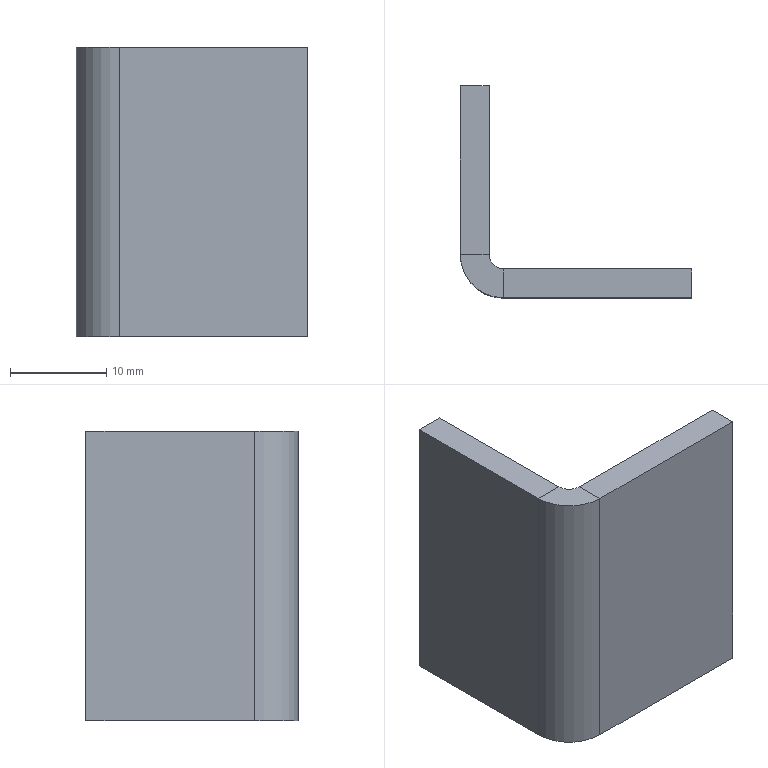Part | STEP file | 5091404 | 1 solid | 14 faces | box 24 x 22 x 30 mm | volume 3754 mm3 | plane 12 | cylinder 2 | commonest cylinder face diameters 3 x1 9 x1
STEP:
#1=CARTESIAN_POINT('',(0.,0.,0.));
#2=DIRECTION('',(0.,0.,1.));
#3=DIRECTION('',(1.,0.,0.));
#4=AXIS2_PLACEMENT_3D('',#1,#2,#3);
#5=CARTESIAN_POINT('',(0.,4.5,15.));
#6=VERTEX_POINT('',#5);
#7=CARTESIAN_POINT('',(3.,4.5,15.));
#8=VERTEX_POINT('',#7);
#9=CARTESIAN_POINT('',(0.,4.5,15.));
#10=DIRECTION('',(1.,0.,0.));
#11=VECTOR('',#10,1.);
#12=LINE('',#9,#11);
#13=CARTESIAN_POINT('',(0.,4.5,15.));
#14=DIRECTION('',(0.,0.,1.));
#15=DIRECTION('',(1.,0.,0.));
#16=AXIS2_PLACEMENT_3D('',#13,#14,#15);
#17=PLANE('',#16);
#18=CARTESIAN_POINT('',(0.,0.));
#19=DIRECTION('',(1.,0.));
#20=VECTOR('',#19,1.);
#21=LINE('',#18,#20);
#22=(GEOMETRIC_REPRESENTATION_CONTEXT(2)PARAMETRIC_REPRESENTATION_CONTEXT()REPRESENTATION_CONTEXT('',''));
#23=DEFINITIONAL_REPRESENTATION('',(#21),#22);
#24=PCURVE('',#17,#23);
#25=CARTESIAN_POINT('',(4.5,3.,15.));
#26=DIRECTION('',(0.,0.,1.));
#27=DIRECTION('',(1.,0.,0.));
#28=AXIS2_PLACEMENT_3D('',#25,#26,#27);
#29=PLANE('',#28);
#30=CARTESIAN_POINT('',(-4.5,1.5));
#31=DIRECTION('',(1.,0.));
#32=VECTOR('',#31,1.);
#33=LINE('',#30,#32);
#34=(GEOMETRIC_REPRESENTATION_CONTEXT(2)PARAMETRIC_REPRESENTATION_CONTEXT()REPRESENTATION_CONTEXT('',''));
#35=DEFINITIONAL_REPRESENTATION('',(#33),#34);
#36=PCURVE('',#29,#35);
#37=SURFACE_CURVE('',#12,(#24,#36),.PCURVE_S1.);
#38=EDGE_CURVE('',#6,#8,#37,.T.);
#39=ORIENTED_EDGE('',*,*,#38,.F.);
#40=CARTESIAN_POINT('',(4.5,0.,15.));
#41=VERTEX_POINT('',#40);
#42=CARTESIAN_POINT('',(4.5,4.5,15.));
#43=DIRECTION('',(0.,0.,1.));
#44=DIRECTION('',(-1.,0.,0.));
#45=AXIS2_PLACEMENT_3D('',#42,#43,#44);
#46=CIRCLE('',#45,4.5);
#47=CARTESIAN_POINT('',(4.5,0.));
#48=DIRECTION('',(-1.,0.));
#49=AXIS2_PLACEMENT_2D('',#47,#48);
#50=CIRCLE('',#49,4.5);
#51=(GEOMETRIC_REPRESENTATION_CONTEXT(2)PARAMETRIC_REPRESENTATION_CONTEXT()REPRESENTATION_CONTEXT('',''));
#52=DEFINITIONAL_REPRESENTATION('',(#50),#51);
#53=PCURVE('',#17,#52);
#54=CARTESIAN_POINT('',(4.5,4.5,15.));
#55=DIRECTION('',(0.,0.,-1.));
#56=DIRECTION('',(-1.,0.,0.));
#57=AXIS2_PLACEMENT_3D('',#54,#55,#56);
#58=CYLINDRICAL_SURFACE('',#57,4.5);
#59=CARTESIAN_POINT('',(6.283,0.));
#60=DIRECTION('',(-1.,0.));
#61=VECTOR('',#60,1.);
#62=LINE('',#59,#61);
#63=(GEOMETRIC_REPRESENTATION_CONTEXT(2)PARAMETRIC_REPRESENTATION_CONTEXT()REPRESENTATION_CONTEXT('',''));
#64=DEFINITIONAL_REPRESENTATION('',(#62),#63);
#65=PCURVE('',#58,#64);
#66=SURFACE_CURVE('',#46,(#53,#65),.PCURVE_S1.);
#67=EDGE_CURVE('',#6,#41,#66,.T.);
#68=ORIENTED_EDGE('',*,*,#67,.T.);
#69=CARTESIAN_POINT('',(4.5,3.,15.));
#70=VERTEX_POINT('',#69);
#71=CARTESIAN_POINT('',(4.5,3.,15.));
#72=DIRECTION('',(0.,-1.,0.));
#73=VECTOR('',#72,1.);
#74=LINE('',#71,#73);
#75=CARTESIAN_POINT('',(4.5,-1.5));
#76=DIRECTION('',(0.,-1.));
#77=VECTOR('',#76,1.);
#78=LINE('',#75,#77);
#79=(GEOMETRIC_REPRESENTATION_CONTEXT(2)PARAMETRIC_REPRESENTATION_CONTEXT()REPRESENTATION_CONTEXT('',''));
#80=DEFINITIONAL_REPRESENTATION('',(#78),#79);
#81=PCURVE('',#17,#80);
#82=CARTESIAN_POINT('',(4.5,4.5,15.));
#83=DIRECTION('',(0.,0.,1.));
#84=DIRECTION('',(1.,0.,0.));
#85=AXIS2_PLACEMENT_3D('',#82,#83,#84);
#86=PLANE('',#85);
#87=CARTESIAN_POINT('',(0.,-1.5));
#88=DIRECTION('',(0.,-1.));
#89=VECTOR('',#88,1.);
#90=LINE('',#87,#89);
#91=(GEOMETRIC_REPRESENTATION_CONTEXT(2)PARAMETRIC_REPRESENTATION_CONTEXT()REPRESENTATION_CONTEXT('',''));
#92=DEFINITIONAL_REPRESENTATION('',(#90),#91);
#93=PCURVE('',#86,#92);
#94=SURFACE_CURVE('',#74,(#81,#93),.PCURVE_S1.);
#95=EDGE_CURVE('',#70,#41,#94,.T.);
#96=ORIENTED_EDGE('',*,*,#95,.F.);
#97=CARTESIAN_POINT('',(4.5,4.5,15.));
#98=DIRECTION('',(0.,0.,1.));
#99=DIRECTION('',(1.,0.,0.));
#100=AXIS2_PLACEMENT_3D('',#97,#98,#99);
#101=CIRCLE('',#100,1.5);
#102=CARTESIAN_POINT('',(4.5,0.));
#103=DIRECTION('',(1.,0.));
#104=AXIS2_PLACEMENT_2D('',#102,#103);
#105=CIRCLE('',#104,1.5);
#106=(GEOMETRIC_REPRESENTATION_CONTEXT(2)PARAMETRIC_REPRESENTATION_CONTEXT()REPRESENTATION_CONTEXT('',''));
#107=DEFINITIONAL_REPRESENTATION('',(#105),#106);
#108=PCURVE('',#17,#107);
#109=CARTESIAN_POINT('',(4.5,4.5,15.));
#110=DIRECTION('',(0.,0.,-1.));
#111=DIRECTION('',(-1.,0.,0.));
#112=AXIS2_PLACEMENT_3D('',#109,#110,#111);
#113=CYLINDRICAL_SURFACE('',#112,1.5);
#114=CARTESIAN_POINT('',(9.425,0.));
#115=DIRECTION('',(-1.,0.));
#116=VECTOR('',#115,1.);
#117=LINE('',#114,#116);
#118=(GEOMETRIC_REPRESENTATION_CONTEXT(2)PARAMETRIC_REPRESENTATION_CONTEXT()REPRESENTATION_CONTEXT('',''));
#119=DEFINITIONAL_REPRESENTATION('',(#117),#118);
#120=PCURVE('',#113,#119);
#121=SURFACE_CURVE('',#101,(#108,#120),.PCURVE_S1.);
#122=EDGE_CURVE('',#8,#70,#121,.T.);
#123=ORIENTED_EDGE('',*,*,#122,.F.);
#124=EDGE_LOOP('',(#39,#68,#96,#123));
#125=FACE_BOUND('',#124,.T.);
#126=ADVANCED_FACE('',(#125),#17,.T.);
#127=CARTESIAN_POINT('',(0.,22.,15.));
#128=VERTEX_POINT('',#127);
#129=CARTESIAN_POINT('',(0.,0.,15.));
#130=DIRECTION('',(0.,-1.,0.));
#131=VECTOR('',#130,1.);
#132=LINE('',#129,#131);
#133=CARTESIAN_POINT('',(-4.5,-3.));
#134=DIRECTION('',(0.,-1.));
#135=VECTOR('',#134,1.);
#136=LINE('',#133,#135);
#137=(GEOMETRIC_REPRESENTATION_CONTEXT(2)PARAMETRIC_REPRESENTATION_CONTEXT()REPRESENTATION_CONTEXT('',''));
#138=DEFINITIONAL_REPRESENTATION('',(#136),#137);
#139=PCURVE('',#29,#138);
#140=CARTESIAN_POINT('',(0.,0.,15.));
#141=DIRECTION('',(1.,0.,0.));
#142=DIRECTION('',(0.,0.,-1.));
#143=AXIS2_PLACEMENT_3D('',#140,#141,#142);
#144=PLANE('',#143);
#145=CARTESIAN_POINT('',(0.,0.));
#146=DIRECTION('',(0.,-1.));
#147=VECTOR('',#146,1.);
#148=LINE('',#145,#147);
#149=(GEOMETRIC_REPRESENTATION_CONTEXT(2)PARAMETRIC_REPRESENTATION_CONTEXT()REPRESENTATION_CONTEXT('',''));
#150=DEFINITIONAL_REPRESENTATION('',(#148),#149);
#151=PCURVE('',#144,#150);
#152=SURFACE_CURVE('',#132,(#139,#151),.PCURVE_S1.);
#153=EDGE_CURVE('',#128,#6,#152,.T.);
#154=ORIENTED_EDGE('',*,*,#153,.T.);
#155=ORIENTED_EDGE('',*,*,#38,.T.);
#156=CARTESIAN_POINT('',(3.,22.,15.));
#157=VERTEX_POINT('',#156);
#158=CARTESIAN_POINT('',(3.,0.,15.));
#159=DIRECTION('',(0.,-1.,0.));
#160=VECTOR('',#159,1.);
#161=LINE('',#158,#160);
#162=CARTESIAN_POINT('',(-1.5,-3.));
#163=DIRECTION('',(0.,-1.));
#164=VECTOR('',#163,1.);
#165=LINE('',#162,#164);
#166=(GEOMETRIC_REPRESENTATION_CONTEXT(2)PARAMETRIC_REPRESENTATION_CONTEXT()REPRESENTATION_CONTEXT('',''));
#167=DEFINITIONAL_REPRESENTATION('',(#165),#166);
#168=PCURVE('',#29,#167);
#169=CARTESIAN_POINT('',(3.,0.,15.));
#170=DIRECTION('',(1.,0.,0.));
#171=DIRECTION('',(0.,0.,-1.));
#172=AXIS2_PLACEMENT_3D('',#169,#170,#171);
#173=PLANE('',#172);
#174=CARTESIAN_POINT('',(0.,0.));
#175=DIRECTION('',(0.,-1.));
#176=VECTOR('',#175,1.);
#177=LINE('',#174,#176);
#178=(GEOMETRIC_REPRESENTATION_CONTEXT(2)PARAMETRIC_REPRESENTATION_CONTEXT()REPRESENTATION_CONTEXT('',''));
#179=DEFINITIONAL_REPRESENTATION('',(#177),#178);
#180=PCURVE('',#173,#179);
#181=SURFACE_CURVE('',#161,(#168,#180),.PCURVE_S1.);
#182=EDGE_CURVE('',#157,#8,#181,.T.);
#183=ORIENTED_EDGE('',*,*,#182,.F.);
#184=CARTESIAN_POINT('',(0.,22.,15.));
#185=DIRECTION('',(1.,0.,0.));
#186=VECTOR('',#185,1.);
#187=LINE('',#184,#186);
#188=CARTESIAN_POINT('',(-4.5,19.));
#189=DIRECTION('',(1.,0.));
#190=VECTOR('',#189,1.);
#191=LINE('',#188,#190);
#192=(GEOMETRIC_REPRESENTATION_CONTEXT(2)PARAMETRIC_REPRESENTATION_CONTEXT()REPRESENTATION_CONTEXT('',''));
#193=DEFINITIONAL_REPRESENTATION('',(#191),#192);
#194=PCURVE('',#29,#193);
#195=CARTESIAN_POINT('',(0.,22.,15.));
#196=DIRECTION('',(0.,1.,0.));
#197=DIRECTION('',(0.,0.,1.));
#198=AXIS2_PLACEMENT_3D('',#195,#196,#197);
#199=PLANE('',#198);
#200=CARTESIAN_POINT('',(0.,0.));
#201=DIRECTION('',(0.,1.));
#202=VECTOR('',#201,1.);
#203=LINE('',#200,#202);
#204=(GEOMETRIC_REPRESENTATION_CONTEXT(2)PARAMETRIC_REPRESENTATION_CONTEXT()REPRESENTATION_CONTEXT('',''));
#205=DEFINITIONAL_REPRESENTATION('',(#203),#204);
#206=PCURVE('',#199,#205);
#207=SURFACE_CURVE('',#187,(#194,#206),.PCURVE_S1.);
#208=EDGE_CURVE('',#128,#157,#207,.T.);
#209=ORIENTED_EDGE('',*,*,#208,.F.);
#210=EDGE_LOOP('',(#154,#155,#183,#209));
#211=FACE_BOUND('',#210,.T.);
#212=ADVANCED_FACE('',(#211),#29,.T.);
#213=CARTESIAN_POINT('',(4.5,0.,-15.));
#214=VERTEX_POINT('',#213);
#215=CARTESIAN_POINT('',(4.5,3.,-15.));
#216=VERTEX_POINT('',#215);
#217=CARTESIAN_POINT('',(4.5,0.,-15.));
#218=DIRECTION('',(0.,1.,0.));
#219=VECTOR('',#218,1.);
#220=LINE('',#217,#219);
#221=CARTESIAN_POINT('',(4.5,0.,-15.));
#222=DIRECTION('',(0.,0.,-1.));
#223=DIRECTION('',(-1.,0.,0.));
#224=AXIS2_PLACEMENT_3D('',#221,#222,#223);
#225=PLANE('',#224);
#226=CARTESIAN_POINT('',(0.,0.));
#227=DIRECTION('',(0.,1.));
#228=VECTOR('',#227,1.);
#229=LINE('',#226,#228);
#230=(GEOMETRIC_REPRESENTATION_CONTEXT(2)PARAMETRIC_REPRESENTATION_CONTEXT()REPRESENTATION_CONTEXT('',''));
#231=DEFINITIONAL_REPRESENTATION('',(#229),#230);
#232=PCURVE('',#225,#231);
#233=CARTESIAN_POINT('',(3.,4.5,-15.));
#234=DIRECTION('',(0.,0.,-1.));
#235=DIRECTION('',(-1.,0.,0.));
#236=AXIS2_PLACEMENT_3D('',#233,#234,#235);
#237=PLANE('',#236);
#238=CARTESIAN_POINT('',(-1.5,-4.5));
#239=DIRECTION('',(0.,1.));
#240=VECTOR('',#239,1.);
#241=LINE('',#238,#240);
#242=(GEOMETRIC_REPRESENTATION_CONTEXT(2)PARAMETRIC_REPRESENTATION_CONTEXT()REPRESENTATION_CONTEXT('',''));
#243=DEFINITIONAL_REPRESENTATION('',(#241),#242);
#244=PCURVE('',#237,#243);
#245=SURFACE_CURVE('',#220,(#232,#244),.PCURVE_S1.);
#246=EDGE_CURVE('',#214,#216,#245,.T.);
#247=ORIENTED_EDGE('',*,*,#246,.F.);
#248=CARTESIAN_POINT('',(0.,4.5,-15.));
#249=VERTEX_POINT('',#248);
#250=CARTESIAN_POINT('',(4.5,4.5,-15.));
#251=DIRECTION('',(0.,0.,1.));
#252=DIRECTION('',(-1.,0.,0.));
#253=AXIS2_PLACEMENT_3D('',#250,#251,#252);
#254=CIRCLE('',#253,4.5);
#255=CARTESIAN_POINT('',(4.5,4.5));
#256=CARTESIAN_POINT('',(4.5,-3.294));
#257=CARTESIAN_POINT('',(-2.25,0.6029));
#258=CARTESIAN_POINT('',(-9.,4.5));
#259=CARTESIAN_POINT('',(-2.25,8.397));
#260=CARTESIAN_POINT('',(4.5,12.294));
#261=CARTESIAN_POINT('',(4.5,4.5));
#262=(BOUNDED_CURVE()B_SPLINE_CURVE(2,(#255,#256,#257,#258,#259,#260,#261),.UNSPECIFIED.,.T.,.F.)B_SPLINE_CURVE_WITH_KNOTS((1,2,2,2,2,1),(-2.094,0.,2.094,4.189,6.283,8.378),.UNSPECIFIED.)CURVE()GEOMETRIC_REPRESENTATION_ITEM()RATIONAL_B_SPLINE_CURVE((1.,0.5,1.,0.5,1.,0.5,1.))REPRESENTATION_ITEM(''));
#263=(GEOMETRIC_REPRESENTATION_CONTEXT(2)PARAMETRIC_REPRESENTATION_CONTEXT()REPRESENTATION_CONTEXT('',''));
#264=DEFINITIONAL_REPRESENTATION('',(#262),#263);
#265=PCURVE('',#225,#264);
#266=CARTESIAN_POINT('',(6.283,30.));
#267=DIRECTION('',(-1.,0.));
#268=VECTOR('',#267,1.);
#269=LINE('',#266,#268);
#270=(GEOMETRIC_REPRESENTATION_CONTEXT(2)PARAMETRIC_REPRESENTATION_CONTEXT()REPRESENTATION_CONTEXT('',''));
#271=DEFINITIONAL_REPRESENTATION('',(#269),#270);
#272=PCURVE('',#58,#271);
#273=SURFACE_CURVE('',#254,(#265,#272),.PCURVE_S1.);
#274=EDGE_CURVE('',#249,#214,#273,.T.);
#275=ORIENTED_EDGE('',*,*,#274,.F.);
#276=CARTESIAN_POINT('',(3.,4.5,-15.));
#277=VERTEX_POINT('',#276);
#278=CARTESIAN_POINT('',(3.,4.5,-15.));
#279=DIRECTION('',(-1.,0.,0.));
#280=VECTOR('',#279,1.);
#281=LINE('',#278,#280);
#282=CARTESIAN_POINT('',(1.5,4.5));
#283=DIRECTION('',(1.,0.));
#284=VECTOR('',#283,1.);
#285=LINE('',#282,#284);
#286=(GEOMETRIC_REPRESENTATION_CONTEXT(2)PARAMETRIC_REPRESENTATION_CONTEXT()REPRESENTATION_CONTEXT('',''));
#287=DEFINITIONAL_REPRESENTATION('',(#285),#286);
#288=PCURVE('',#225,#287);
#289=CARTESIAN_POINT('',(4.5,4.5,-15.));
#290=DIRECTION('',(0.,0.,1.));
#291=DIRECTION('',(1.,0.,0.));
#292=AXIS2_PLACEMENT_3D('',#289,#290,#291);
#293=PLANE('',#292);
#294=CARTESIAN_POINT('',(-1.5,0.));
#295=DIRECTION('',(-1.,0.));
#296=VECTOR('',#295,1.);
#297=LINE('',#294,#296);
#298=(GEOMETRIC_REPRESENTATION_CONTEXT(2)PARAMETRIC_REPRESENTATION_CONTEXT()REPRESENTATION_CONTEXT('',''));
#299=DEFINITIONAL_REPRESENTATION('',(#297),#298);
#300=PCURVE('',#293,#299);
#301=SURFACE_CURVE('',#281,(#288,#300),.PCURVE_S1.);
#302=EDGE_CURVE('',#277,#249,#301,.T.);
#303=ORIENTED_EDGE('',*,*,#302,.F.);
#304=CARTESIAN_POINT('',(4.5,4.5,-15.));
#305=DIRECTION('',(0.,0.,1.));
#306=DIRECTION('',(1.,0.,0.));
#307=AXIS2_PLACEMENT_3D('',#304,#305,#306);
#308=CIRCLE('',#307,1.5);
#309=CARTESIAN_POINT('',(-1.5,4.5));
#310=CARTESIAN_POINT('',(-1.5,7.098));
#311=CARTESIAN_POINT('',(0.75,5.799));
#312=CARTESIAN_POINT('',(3.,4.5));
#313=CARTESIAN_POINT('',(0.75,3.201));
#314=CARTESIAN_POINT('',(-1.5,1.902));
#315=CARTESIAN_POINT('',(-1.5,4.5));
#316=(BOUNDED_CURVE()B_SPLINE_CURVE(2,(#309,#310,#311,#312,#313,#314,#315),.UNSPECIFIED.,.T.,.F.)B_SPLINE_CURVE_WITH_KNOTS((1,2,2,2,2,1),(-2.094,0.,2.094,4.189,6.283,8.378),.UNSPECIFIED.)CURVE()GEOMETRIC_REPRESENTATION_ITEM()RATIONAL_B_SPLINE_CURVE((1.,0.5,1.,0.5,1.,0.5,1.))REPRESENTATION_ITEM(''));
#317=(GEOMETRIC_REPRESENTATION_CONTEXT(2)PARAMETRIC_REPRESENTATION_CONTEXT()REPRESENTATION_CONTEXT('',''));
#318=DEFINITIONAL_REPRESENTATION('',(#316),#317);
#319=PCURVE('',#225,#318);
#320=CARTESIAN_POINT('',(9.425,30.));
#321=DIRECTION('',(-1.,0.));
#322=VECTOR('',#321,1.);
#323=LINE('',#320,#322);
#324=(GEOMETRIC_REPRESENTATION_CONTEXT(2)PARAMETRIC_REPRESENTATION_CONTEXT()REPRESENTATION_CONTEXT('',''));
#325=DEFINITIONAL_REPRESENTATION('',(#323),#324);
#326=PCURVE('',#113,#325);
#327=SURFACE_CURVE('',#308,(#319,#326),.PCURVE_S1.);
#328=EDGE_CURVE('',#277,#216,#327,.T.);
#329=ORIENTED_EDGE('',*,*,#328,.T.);
#330=EDGE_LOOP('',(#247,#275,#303,#329));
#331=FACE_BOUND('',#330,.T.);
#332=ADVANCED_FACE('',(#331),#225,.T.);
#333=CARTESIAN_POINT('',(24.,0.,-15.));
#334=VERTEX_POINT('',#333);
#335=CARTESIAN_POINT('',(0.,0.,-15.));
#336=DIRECTION('',(1.,0.,0.));
#337=VECTOR('',#336,1.);
#338=LINE('',#335,#337);
#339=CARTESIAN_POINT('',(3.,-4.5));
#340=DIRECTION('',(-1.,0.));
#341=VECTOR('',#340,1.);
#342=LINE('',#339,#341);
#343=(GEOMETRIC_REPRESENTATION_CONTEXT(2)PARAMETRIC_REPRESENTATION_CONTEXT()REPRESENTATION_CONTEXT('',''));
#344=DEFINITIONAL_REPRESENTATION('',(#342),#343);
#345=PCURVE('',#237,#344);
#346=CARTESIAN_POINT('',(0.,0.,15.));
#347=DIRECTION('',(0.,1.,0.));
#348=DIRECTION('',(0.,0.,1.));
#349=AXIS2_PLACEMENT_3D('',#346,#347,#348);
#350=PLANE('',#349);
#351=CARTESIAN_POINT('',(-30.,0.));
#352=DIRECTION('',(0.,1.));
#353=VECTOR('',#352,1.);
#354=LINE('',#351,#353);
#355=(GEOMETRIC_REPRESENTATION_CONTEXT(2)PARAMETRIC_REPRESENTATION_CONTEXT()REPRESENTATION_CONTEXT('',''));
#356=DEFINITIONAL_REPRESENTATION('',(#354),#355);
#357=PCURVE('',#350,#356);
#358=SURFACE_CURVE('',#338,(#345,#357),.PCURVE_S1.);
#359=EDGE_CURVE('',#214,#334,#358,.T.);
#360=ORIENTED_EDGE('',*,*,#359,.F.);
#361=ORIENTED_EDGE('',*,*,#246,.T.);
#362=CARTESIAN_POINT('',(24.,3.,-15.));
#363=VERTEX_POINT('',#362);
#364=CARTESIAN_POINT('',(0.,3.,-15.));
#365=DIRECTION('',(1.,0.,0.));
#366=VECTOR('',#365,1.);
#367=LINE('',#364,#366);
#368=CARTESIAN_POINT('',(3.,-1.5));
#369=DIRECTION('',(-1.,0.));
#370=VECTOR('',#369,1.);
#371=LINE('',#368,#370);
#372=(GEOMETRIC_REPRESENTATION_CONTEXT(2)PARAMETRIC_REPRESENTATION_CONTEXT()REPRESENTATION_CONTEXT('',''));
#373=DEFINITIONAL_REPRESENTATION('',(#371),#372);
#374=PCURVE('',#237,#373);
#375=CARTESIAN_POINT('',(0.,3.,15.));
#376=DIRECTION('',(0.,1.,0.));
#377=DIRECTION('',(0.,0.,1.));
#378=AXIS2_PLACEMENT_3D('',#375,#376,#377);
#379=PLANE('',#378);
#380=CARTESIAN_POINT('',(-30.,0.));
#381=DIRECTION('',(0.,1.));
#382=VECTOR('',#381,1.);
#383=LINE('',#380,#382);
#384=(GEOMETRIC_REPRESENTATION_CONTEXT(2)PARAMETRIC_REPRESENTATION_CONTEXT()REPRESENTATION_CONTEXT('',''));
#385=DEFINITIONAL_REPRESENTATION('',(#383),#384);
#386=PCURVE('',#379,#385);
#387=SURFACE_CURVE('',#367,(#374,#386),.PCURVE_S1.);
#388=EDGE_CURVE('',#216,#363,#387,.T.);
#389=ORIENTED_EDGE('',*,*,#388,.T.);
#390=CARTESIAN_POINT('',(24.,3.,-15.));
#391=DIRECTION('',(0.,-1.,0.));
#392=VECTOR('',#391,1.);
#393=LINE('',#390,#392);
#394=CARTESIAN_POINT('',(-21.,-1.5));
#395=DIRECTION('',(0.,-1.));
#396=VECTOR('',#395,1.);
#397=LINE('',#394,#396);
#398=(GEOMETRIC_REPRESENTATION_CONTEXT(2)PARAMETRIC_REPRESENTATION_CONTEXT()REPRESENTATION_CONTEXT('',''));
#399=DEFINITIONAL_REPRESENTATION('',(#397),#398);
#400=PCURVE('',#237,#399);
#401=CARTESIAN_POINT('',(24.,3.,15.));
#402=DIRECTION('',(1.,0.,0.));
#403=DIRECTION('',(0.,0.,-1.));
#404=AXIS2_PLACEMENT_3D('',#401,#402,#403);
#405=PLANE('',#404);
#406=CARTESIAN_POINT('',(30.,0.));
#407=DIRECTION('',(0.,-1.));
#408=VECTOR('',#407,1.);
#409=LINE('',#406,#408);
#410=(GEOMETRIC_REPRESENTATION_CONTEXT(2)PARAMETRIC_REPRESENTATION_CONTEXT()REPRESENTATION_CONTEXT('',''));
#411=DEFINITIONAL_REPRESENTATION('',(#409),#410);
#412=PCURVE('',#405,#411);
#413=SURFACE_CURVE('',#393,(#400,#412),.PCURVE_S1.);
#414=EDGE_CURVE('',#363,#334,#413,.T.);
#415=ORIENTED_EDGE('',*,*,#414,.T.);
#416=EDGE_LOOP('',(#360,#361,#389,#415));
#417=FACE_BOUND('',#416,.T.);
#418=ADVANCED_FACE('',(#417),#237,.T.);
#419=ORIENTED_EDGE('',*,*,#359,.T.);
#420=CARTESIAN_POINT('',(24.,0.,15.));
#421=VERTEX_POINT('',#420);
#422=CARTESIAN_POINT('',(24.,0.,15.));
#423=DIRECTION('',(0.,0.,-1.));
#424=VECTOR('',#423,1.);
#425=LINE('',#422,#424);
#426=CARTESIAN_POINT('',(0.,24.));
#427=DIRECTION('',(-1.,0.));
#428=VECTOR('',#427,1.);
#429=LINE('',#426,#428);
#430=(GEOMETRIC_REPRESENTATION_CONTEXT(2)PARAMETRIC_REPRESENTATION_CONTEXT()REPRESENTATION_CONTEXT('',''));
#431=DEFINITIONAL_REPRESENTATION('',(#429),#430);
#432=PCURVE('',#350,#431);
#433=CARTESIAN_POINT('',(0.,-3.));
#434=DIRECTION('',(1.,0.));
#435=VECTOR('',#434,1.);
#436=LINE('',#433,#435);
#437=(GEOMETRIC_REPRESENTATION_CONTEXT(2)PARAMETRIC_REPRESENTATION_CONTEXT()REPRESENTATION_CONTEXT('',''));
#438=DEFINITIONAL_REPRESENTATION('',(#436),#437);
#439=PCURVE('',#405,#438);
#440=SURFACE_CURVE('',#425,(#432,#439),.PCURVE_S1.);
#441=EDGE_CURVE('',#421,#334,#440,.T.);
#442=ORIENTED_EDGE('',*,*,#441,.F.);
#443=CARTESIAN_POINT('',(0.,0.,15.));
#444=DIRECTION('',(1.,0.,0.));
#445=VECTOR('',#444,1.);
#446=LINE('',#443,#445);
#447=CARTESIAN_POINT('',(0.,0.));
#448=DIRECTION('',(0.,1.));
#449=VECTOR('',#448,1.);
#450=LINE('',#447,#449);
#451=(GEOMETRIC_REPRESENTATION_CONTEXT(2)PARAMETRIC_REPRESENTATION_CONTEXT()REPRESENTATION_CONTEXT('',''));
#452=DEFINITIONAL_REPRESENTATION('',(#450),#451);
#453=PCURVE('',#350,#452);
#454=CARTESIAN_POINT('',(-4.5,-4.5));
#455=DIRECTION('',(1.,0.));
#456=VECTOR('',#455,1.);
#457=LINE('',#454,#456);
#458=(GEOMETRIC_REPRESENTATION_CONTEXT(2)PARAMETRIC_REPRESENTATION_CONTEXT()REPRESENTATION_CONTEXT('',''));
#459=DEFINITIONAL_REPRESENTATION('',(#457),#458);
#460=PCURVE('',#86,#459);
#461=SURFACE_CURVE('',#446,(#453,#460),.PCURVE_S1.);
#462=EDGE_CURVE('',#41,#421,#461,.T.);
#463=ORIENTED_EDGE('',*,*,#462,.F.);
#464=CARTESIAN_POINT('',(4.5,0.,15.));
#465=DIRECTION('',(0.,0.,-1.));
#466=VECTOR('',#465,1.);
#467=LINE('',#464,#466);
#468=CARTESIAN_POINT('',(0.,4.5));
#469=DIRECTION('',(-1.,0.));
#470=VECTOR('',#469,1.);
#471=LINE('',#468,#470);
#472=(GEOMETRIC_REPRESENTATION_CONTEXT(2)PARAMETRIC_REPRESENTATION_CONTEXT()REPRESENTATION_CONTEXT('',''));
#473=DEFINITIONAL_REPRESENTATION('',(#471),#472);
#474=PCURVE('',#350,#473);
#475=CARTESIAN_POINT('',(4.712,0.));
#476=DIRECTION('',(0.,1.));
#477=VECTOR('',#476,1.);
#478=LINE('',#475,#477);
#479=(GEOMETRIC_REPRESENTATION_CONTEXT(2)PARAMETRIC_REPRESENTATION_CONTEXT()REPRESENTATION_CONTEXT('',''));
#480=DEFINITIONAL_REPRESENTATION('',(#478),#479);
#481=PCURVE('',#58,#480);
#482=SURFACE_CURVE('',#467,(#474,#481),.PCURVE_S1.);
#483=EDGE_CURVE('',#41,#214,#482,.T.);
#484=ORIENTED_EDGE('',*,*,#483,.T.);
#485=EDGE_LOOP('',(#419,#442,#463,#484));
#486=FACE_BOUND('',#485,.T.);
#487=ADVANCED_FACE('',(#486),#350,.F.);
#488=ORIENTED_EDGE('',*,*,#414,.F.);
#489=CARTESIAN_POINT('',(24.,3.,15.));
#490=VERTEX_POINT('',#489);
#491=CARTESIAN_POINT('',(24.,3.,15.));
#492=DIRECTION('',(0.,0.,-1.));
#493=VECTOR('',#492,1.);
#494=LINE('',#491,#493);
#495=CARTESIAN_POINT('',(0.,0.));
#496=DIRECTION('',(1.,0.));
#497=VECTOR('',#496,1.);
#498=LINE('',#495,#497);
#499=(GEOMETRIC_REPRESENTATION_CONTEXT(2)PARAMETRIC_REPRESENTATION_CONTEXT()REPRESENTATION_CONTEXT('',''));
#500=DEFINITIONAL_REPRESENTATION('',(#498),#499);
#501=PCURVE('',#405,#500);
#502=CARTESIAN_POINT('',(0.,24.));
#503=DIRECTION('',(-1.,0.));
#504=VECTOR('',#503,1.);
#505=LINE('',#502,#504);
#506=(GEOMETRIC_REPRESENTATION_CONTEXT(2)PARAMETRIC_REPRESENTATION_CONTEXT()REPRESENTATION_CONTEXT('',''));
#507=DEFINITIONAL_REPRESENTATION('',(#505),#506);
#508=PCURVE('',#379,#507);
#509=SURFACE_CURVE('',#494,(#501,#508),.PCURVE_S1.);
#510=EDGE_CURVE('',#490,#363,#509,.T.);
#511=ORIENTED_EDGE('',*,*,#510,.F.);
#512=CARTESIAN_POINT('',(24.,3.,15.));
#513=DIRECTION('',(0.,-1.,0.));
#514=VECTOR('',#513,1.);
#515=LINE('',#512,#514);
#516=CARTESIAN_POINT('',(0.,0.));
#517=DIRECTION('',(0.,-1.));
#518=VECTOR('',#517,1.);
#519=LINE('',#516,#518);
#520=(GEOMETRIC_REPRESENTATION_CONTEXT(2)PARAMETRIC_REPRESENTATION_CONTEXT()REPRESENTATION_CONTEXT('',''));
#521=DEFINITIONAL_REPRESENTATION('',(#519),#520);
#522=PCURVE('',#405,#521);
#523=CARTESIAN_POINT('',(19.5,-1.5));
#524=DIRECTION('',(0.,-1.));
#525=VECTOR('',#524,1.);
#526=LINE('',#523,#525);
#527=(GEOMETRIC_REPRESENTATION_CONTEXT(2)PARAMETRIC_REPRESENTATION_CONTEXT()REPRESENTATION_CONTEXT('',''));
#528=DEFINITIONAL_REPRESENTATION('',(#526),#527);
#529=PCURVE('',#86,#528);
#530=SURFACE_CURVE('',#515,(#522,#529),.PCURVE_S1.);
#531=EDGE_CURVE('',#490,#421,#530,.T.);
#532=ORIENTED_EDGE('',*,*,#531,.T.);
#533=ORIENTED_EDGE('',*,*,#441,.T.);
#534=EDGE_LOOP('',(#488,#511,#532,#533));
#535=FACE_BOUND('',#534,.T.);
#536=ADVANCED_FACE('',(#535),#405,.T.);
#537=ORIENTED_EDGE('',*,*,#388,.F.);
#538=CARTESIAN_POINT('',(4.5,3.,15.));
#539=DIRECTION('',(0.,0.,-1.));
#540=VECTOR('',#539,1.);
#541=LINE('',#538,#540);
#542=CARTESIAN_POINT('',(0.,4.5));
#543=DIRECTION('',(-1.,0.));
#544=VECTOR('',#543,1.);
#545=LINE('',#542,#544);
#546=(GEOMETRIC_REPRESENTATION_CONTEXT(2)PARAMETRIC_REPRESENTATION_CONTEXT()REPRESENTATION_CONTEXT('',''));
#547=DEFINITIONAL_REPRESENTATION('',(#545),#546);
#548=PCURVE('',#379,#547);
#549=CARTESIAN_POINT('',(4.712,0.));
#550=DIRECTION('',(0.,1.));
#551=VECTOR('',#550,1.);
#552=LINE('',#549,#551);
#553=(GEOMETRIC_REPRESENTATION_CONTEXT(2)PARAMETRIC_REPRESENTATION_CONTEXT()REPRESENTATION_CONTEXT('',''));
#554=DEFINITIONAL_REPRESENTATION('',(#552),#553);
#555=PCURVE('',#113,#554);
#556=SURFACE_CURVE('',#541,(#548,#555),.PCURVE_S1.);
#557=EDGE_CURVE('',#70,#216,#556,.T.);
#558=ORIENTED_EDGE('',*,*,#557,.F.);
#559=CARTESIAN_POINT('',(0.,3.,15.));
#560=DIRECTION('',(1.,0.,0.));
#561=VECTOR('',#560,1.);
#562=LINE('',#559,#561);
#563=CARTESIAN_POINT('',(0.,0.));
#564=DIRECTION('',(0.,1.));
#565=VECTOR('',#564,1.);
#566=LINE('',#563,#565);
#567=(GEOMETRIC_REPRESENTATION_CONTEXT(2)PARAMETRIC_REPRESENTATION_CONTEXT()REPRESENTATION_CONTEXT('',''));
#568=DEFINITIONAL_REPRESENTATION('',(#566),#567);
#569=PCURVE('',#379,#568);
#570=CARTESIAN_POINT('',(-4.5,-1.5));
#571=DIRECTION('',(1.,0.));
#572=VECTOR('',#571,1.);
#573=LINE('',#570,#572);
#574=(GEOMETRIC_REPRESENTATION_CONTEXT(2)PARAMETRIC_REPRESENTATION_CONTEXT()REPRESENTATION_CONTEXT('',''));
#575=DEFINITIONAL_REPRESENTATION('',(#573),#574);
#576=PCURVE('',#86,#575);
#577=SURFACE_CURVE('',#562,(#569,#576),.PCURVE_S1.);
#578=EDGE_CURVE('',#70,#490,#577,.T.);
#579=ORIENTED_EDGE('',*,*,#578,.T.);
#580=ORIENTED_EDGE('',*,*,#510,.T.);
#581=EDGE_LOOP('',(#537,#558,#579,#580));
#582=FACE_BOUND('',#581,.T.);
#583=ADVANCED_FACE('',(#582),#379,.T.);
#584=ORIENTED_EDGE('',*,*,#557,.F.);
#585=ORIENTED_EDGE('',*,*,#122,.F.);
#586=CARTESIAN_POINT('',(3.,4.5,15.));
#587=DIRECTION('',(0.,0.,-1.));
#588=VECTOR('',#587,1.);
#589=LINE('',#586,#588);
#590=CARTESIAN_POINT('',(6.283,0.));
#591=DIRECTION('',(0.,1.));
#592=VECTOR('',#591,1.);
#593=LINE('',#590,#592);
#594=(GEOMETRIC_REPRESENTATION_CONTEXT(2)PARAMETRIC_REPRESENTATION_CONTEXT()REPRESENTATION_CONTEXT('',''));
#595=DEFINITIONAL_REPRESENTATION('',(#593),#594);
#596=PCURVE('',#113,#595);
#597=CARTESIAN_POINT('',(0.,4.5));
#598=DIRECTION('',(1.,0.));
#599=VECTOR('',#598,1.);
#600=LINE('',#597,#599);
#601=(GEOMETRIC_REPRESENTATION_CONTEXT(2)PARAMETRIC_REPRESENTATION_CONTEXT()REPRESENTATION_CONTEXT('',''));
#602=DEFINITIONAL_REPRESENTATION('',(#600),#601);
#603=PCURVE('',#173,#602);
#604=SURFACE_CURVE('',#589,(#596,#603),.PCURVE_S1.);
#605=EDGE_CURVE('',#8,#277,#604,.T.);
#606=ORIENTED_EDGE('',*,*,#605,.T.);
#607=ORIENTED_EDGE('',*,*,#328,.T.);
#608=EDGE_LOOP('',(#584,#585,#606,#607));
#609=FACE_BOUND('',#608,.F.);
#610=ADVANCED_FACE('',(#609),#113,.F.);
#611=CARTESIAN_POINT('',(3.,22.,-15.));
#612=VERTEX_POINT('',#611);
#613=CARTESIAN_POINT('',(3.,0.,-15.));
#614=DIRECTION('',(0.,-1.,0.));
#615=VECTOR('',#614,1.);
#616=LINE('',#613,#615);
#617=CARTESIAN_POINT('',(30.,0.));
#618=DIRECTION('',(0.,-1.));
#619=VECTOR('',#618,1.);
#620=LINE('',#617,#619);
#621=(GEOMETRIC_REPRESENTATION_CONTEXT(2)PARAMETRIC_REPRESENTATION_CONTEXT()REPRESENTATION_CONTEXT('',''));
#622=DEFINITIONAL_REPRESENTATION('',(#620),#621);
#623=PCURVE('',#173,#622);
#624=CARTESIAN_POINT('',(-1.5,-4.5));
#625=DIRECTION('',(0.,-1.));
#626=VECTOR('',#625,1.);
#627=LINE('',#624,#626);
#628=(GEOMETRIC_REPRESENTATION_CONTEXT(2)PARAMETRIC_REPRESENTATION_CONTEXT()REPRESENTATION_CONTEXT('',''));
#629=DEFINITIONAL_REPRESENTATION('',(#627),#628);
#630=PCURVE('',#293,#629);
#631=SURFACE_CURVE('',#616,(#623,#630),.PCURVE_S1.);
#632=EDGE_CURVE('',#612,#277,#631,.T.);
#633=ORIENTED_EDGE('',*,*,#632,.F.);
#634=CARTESIAN_POINT('',(3.,22.,15.));
#635=DIRECTION('',(0.,0.,-1.));
#636=VECTOR('',#635,1.);
#637=LINE('',#634,#636);
#638=CARTESIAN_POINT('',(0.,22.));
#639=DIRECTION('',(1.,0.));
#640=VECTOR('',#639,1.);
#641=LINE('',#638,#640);
#642=(GEOMETRIC_REPRESENTATION_CONTEXT(2)PARAMETRIC_REPRESENTATION_CONTEXT()REPRESENTATION_CONTEXT('',''));
#643=DEFINITIONAL_REPRESENTATION('',(#641),#642);
#644=PCURVE('',#173,#643);
#645=CARTESIAN_POINT('',(0.,3.));
#646=DIRECTION('',(-1.,0.));
#647=VECTOR('',#646,1.);
#648=LINE('',#645,#647);
#649=(GEOMETRIC_REPRESENTATION_CONTEXT(2)PARAMETRIC_REPRESENTATION_CONTEXT()REPRESENTATION_CONTEXT('',''));
#650=DEFINITIONAL_REPRESENTATION('',(#648),#649);
#651=PCURVE('',#199,#650);
#652=SURFACE_CURVE('',#637,(#644,#651),.PCURVE_S1.);
#653=EDGE_CURVE('',#157,#612,#652,.T.);
#654=ORIENTED_EDGE('',*,*,#653,.F.);
#655=ORIENTED_EDGE('',*,*,#182,.T.);
#656=ORIENTED_EDGE('',*,*,#605,.T.);
#657=EDGE_LOOP('',(#633,#654,#655,#656));
#658=FACE_BOUND('',#657,.T.);
#659=ADVANCED_FACE('',(#658),#173,.T.);
#660=CARTESIAN_POINT('',(0.,22.,-15.));
#661=VERTEX_POINT('',#660);
#662=CARTESIAN_POINT('',(0.,22.,-15.));
#663=DIRECTION('',(1.,0.,0.));
#664=VECTOR('',#663,1.);
#665=LINE('',#662,#664);
#666=CARTESIAN_POINT('',(-30.,0.));
#667=DIRECTION('',(0.,1.));
#668=VECTOR('',#667,1.);
#669=LINE('',#666,#668);
#670=(GEOMETRIC_REPRESENTATION_CONTEXT(2)PARAMETRIC_REPRESENTATION_CONTEXT()REPRESENTATION_CONTEXT('',''));
#671=DEFINITIONAL_REPRESENTATION('',(#669),#670);
#672=PCURVE('',#199,#671);
#673=CARTESIAN_POINT('',(-4.5,17.5));
#674=DIRECTION('',(1.,0.));
#675=VECTOR('',#674,1.);
#676=LINE('',#673,#675);
#677=(GEOMETRIC_REPRESENTATION_CONTEXT(2)PARAMETRIC_REPRESENTATION_CONTEXT()REPRESENTATION_CONTEXT('',''));
#678=DEFINITIONAL_REPRESENTATION('',(#676),#677);
#679=PCURVE('',#293,#678);
#680=SURFACE_CURVE('',#665,(#672,#679),.PCURVE_S1.);
#681=EDGE_CURVE('',#661,#612,#680,.T.);
#682=ORIENTED_EDGE('',*,*,#681,.F.);
#683=CARTESIAN_POINT('',(0.,22.,15.));
#684=DIRECTION('',(0.,0.,-1.));
#685=VECTOR('',#684,1.);
#686=LINE('',#683,#685);
#687=CARTESIAN_POINT('',(0.,0.));
#688=DIRECTION('',(-1.,0.));
#689=VECTOR('',#688,1.);
#690=LINE('',#687,#689);
#691=(GEOMETRIC_REPRESENTATION_CONTEXT(2)PARAMETRIC_REPRESENTATION_CONTEXT()REPRESENTATION_CONTEXT('',''));
#692=DEFINITIONAL_REPRESENTATION('',(#690),#691);
#693=PCURVE('',#199,#692);
#694=CARTESIAN_POINT('',(0.,22.));
#695=DIRECTION('',(1.,0.));
#696=VECTOR('',#695,1.);
#697=LINE('',#694,#696);
#698=(GEOMETRIC_REPRESENTATION_CONTEXT(2)PARAMETRIC_REPRESENTATION_CONTEXT()REPRESENTATION_CONTEXT('',''));
#699=DEFINITIONAL_REPRESENTATION('',(#697),#698);
#700=PCURVE('',#144,#699);
#701=SURFACE_CURVE('',#686,(#693,#700),.PCURVE_S1.);
#702=EDGE_CURVE('',#128,#661,#701,.T.);
#703=ORIENTED_EDGE('',*,*,#702,.F.);
#704=ORIENTED_EDGE('',*,*,#208,.T.);
#705=ORIENTED_EDGE('',*,*,#653,.T.);
#706=EDGE_LOOP('',(#682,#703,#704,#705));
#707=FACE_BOUND('',#706,.T.);
#708=ADVANCED_FACE('',(#707),#199,.T.);
#709=CARTESIAN_POINT('',(0.,0.,-15.));
#710=DIRECTION('',(0.,-1.,0.));
#711=VECTOR('',#710,1.);
#712=LINE('',#709,#711);
#713=CARTESIAN_POINT('',(30.,0.));
#714=DIRECTION('',(0.,-1.));
#715=VECTOR('',#714,1.);
#716=LINE('',#713,#715);
#717=(GEOMETRIC_REPRESENTATION_CONTEXT(2)PARAMETRIC_REPRESENTATION_CONTEXT()REPRESENTATION_CONTEXT('',''));
#718=DEFINITIONAL_REPRESENTATION('',(#716),#717);
#719=PCURVE('',#144,#718);
#720=CARTESIAN_POINT('',(-4.5,-4.5));
#721=DIRECTION('',(0.,-1.));
#722=VECTOR('',#721,1.);
#723=LINE('',#720,#722);
#724=(GEOMETRIC_REPRESENTATION_CONTEXT(2)PARAMETRIC_REPRESENTATION_CONTEXT()REPRESENTATION_CONTEXT('',''));
#725=DEFINITIONAL_REPRESENTATION('',(#723),#724);
#726=PCURVE('',#293,#725);
#727=SURFACE_CURVE('',#712,(#719,#726),.PCURVE_S1.);
#728=EDGE_CURVE('',#661,#249,#727,.T.);
#729=ORIENTED_EDGE('',*,*,#728,.T.);
#730=CARTESIAN_POINT('',(0.,4.5,15.));
#731=DIRECTION('',(0.,0.,-1.));
#732=VECTOR('',#731,1.);
#733=LINE('',#730,#732);
#734=CARTESIAN_POINT('',(0.,4.5));
#735=DIRECTION('',(1.,0.));
#736=VECTOR('',#735,1.);
#737=LINE('',#734,#736);
#738=(GEOMETRIC_REPRESENTATION_CONTEXT(2)PARAMETRIC_REPRESENTATION_CONTEXT()REPRESENTATION_CONTEXT('',''));
#739=DEFINITIONAL_REPRESENTATION('',(#737),#738);
#740=PCURVE('',#144,#739);
#741=CARTESIAN_POINT('',(6.283,0.));
#742=DIRECTION('',(0.,1.));
#743=VECTOR('',#742,1.);
#744=LINE('',#741,#743);
#745=(GEOMETRIC_REPRESENTATION_CONTEXT(2)PARAMETRIC_REPRESENTATION_CONTEXT()REPRESENTATION_CONTEXT('',''));
#746=DEFINITIONAL_REPRESENTATION('',(#744),#745);
#747=PCURVE('',#58,#746);
#748=SURFACE_CURVE('',#733,(#740,#747),.PCURVE_S1.);
#749=EDGE_CURVE('',#6,#249,#748,.T.);
#750=ORIENTED_EDGE('',*,*,#749,.F.);
#751=ORIENTED_EDGE('',*,*,#153,.F.);
#752=ORIENTED_EDGE('',*,*,#702,.T.);
#753=EDGE_LOOP('',(#729,#750,#751,#752));
#754=FACE_BOUND('',#753,.T.);
#755=ADVANCED_FACE('',(#754),#144,.F.);
#756=ORIENTED_EDGE('',*,*,#274,.T.);
#757=ORIENTED_EDGE('',*,*,#483,.F.);
#758=ORIENTED_EDGE('',*,*,#67,.F.);
#759=ORIENTED_EDGE('',*,*,#749,.T.);
#760=EDGE_LOOP('',(#756,#757,#758,#759));
#761=FACE_BOUND('',#760,.T.);
#762=ADVANCED_FACE('',(#761),#58,.T.);
#763=ORIENTED_EDGE('',*,*,#462,.T.);
#764=ORIENTED_EDGE('',*,*,#531,.F.);
#765=ORIENTED_EDGE('',*,*,#578,.F.);
#766=ORIENTED_EDGE('',*,*,#95,.T.);
#767=EDGE_LOOP('',(#763,#764,#765,#766));
#768=FACE_BOUND('',#767,.T.);
#769=ADVANCED_FACE('',(#768),#86,.T.);
#770=ORIENTED_EDGE('',*,*,#632,.T.);
#771=ORIENTED_EDGE('',*,*,#302,.T.);
#772=ORIENTED_EDGE('',*,*,#728,.F.);
#773=ORIENTED_EDGE('',*,*,#681,.T.);
#774=EDGE_LOOP('',(#770,#771,#772,#773));
#775=FACE_BOUND('',#774,.T.);
#776=ADVANCED_FACE('',(#775),#293,.F.);
#777=CLOSED_SHELL('',(#126,#212,#332,#418,#487,#536,#583,#610,#659,#708,#755,#762,#769,#776));
#778=MANIFOLD_SOLID_BREP('',#777);
#779=(LENGTH_UNIT()NAMED_UNIT(*)SI_UNIT(.MILLI.,.METRE.));
#780=UNCERTAINTY_MEASURE_WITH_UNIT(LENGTH_MEASURE(0.0000001),#779,'','');
#781=(NAMED_UNIT(*)PLANE_ANGLE_UNIT()SI_UNIT($,.RADIAN.));
#782=(NAMED_UNIT(*)SI_UNIT($,.STERADIAN.)SOLID_ANGLE_UNIT());
#783=(GEOMETRIC_REPRESENTATION_CONTEXT(3)GLOBAL_UNCERTAINTY_ASSIGNED_CONTEXT((#780))GLOBAL_UNIT_ASSIGNED_CONTEXT((#779,#781,#782))REPRESENTATION_CONTEXT('',''));
#784=ADVANCED_BREP_SHAPE_REPRESENTATION('',(#4,#778),#783);